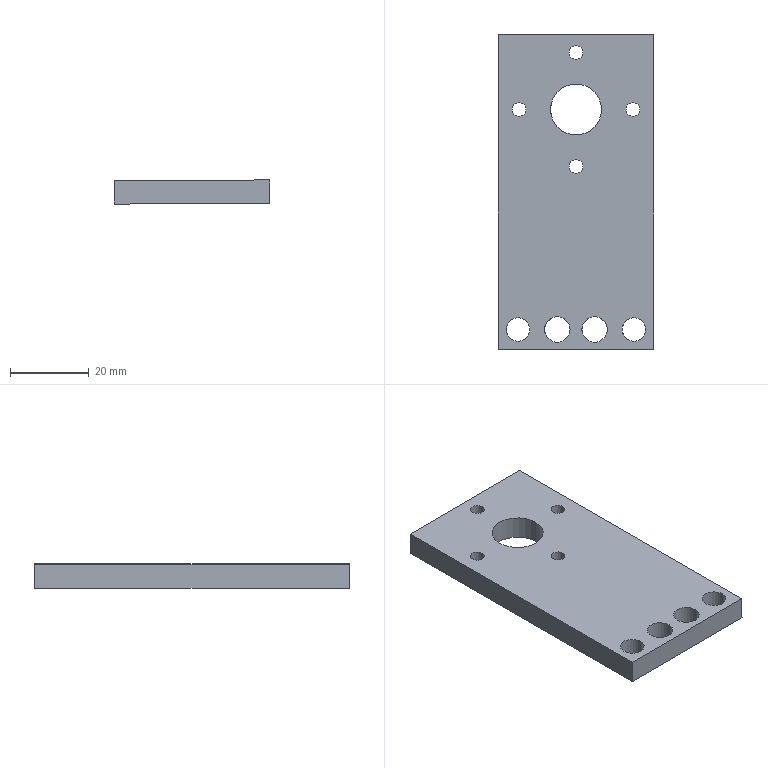Part | SolidWorks | features Cut 2, HoleWzd 2, Extrusion 1 | 1 solid | 24 faces | box 39.504 x 80 x 6.135 mm | volume 17187 mm3 | cylinder 18 | plane 6 | commonest cylinder face diameters 3.5 x8 6 x4 6.5 x4 13 x2
STEP:
#1=CARTESIAN_POINT('',(-183.995,65.629,-9.921));
#2=VERTEX_POINT('',#1);
#3=CARTESIAN_POINT('',(-187.495,65.629,-9.933));
#4=VERTEX_POINT('',#3);
#5=CARTESIAN_POINT('',(-185.745,65.629,-9.927));
#6=DIRECTION('',(0.003428,0.,-1.));
#7=DIRECTION('',(-1.,0.,-0.003428));
#8=AXIS2_PLACEMENT_3D('',#5,#6,#7);
#9=CIRCLE('',#8,1.75);
#10=EDGE_CURVE('',#2,#4,#9,.T.);
#11=ORIENTED_EDGE('',*,*,#10,.T.);
#12=CARTESIAN_POINT('',(-187.515,65.629,-3.933));
#13=VERTEX_POINT('',#12);
#14=CARTESIAN_POINT('',(-187.515,65.629,-3.933));
#15=DIRECTION('',(-0.003428,0.,1.));
#16=VECTOR('',#15,1000.);
#17=LINE('',#14,#16);
#18=EDGE_CURVE('',#4,#13,#17,.T.);
#19=ORIENTED_EDGE('',*,*,#18,.T.);
#20=CARTESIAN_POINT('',(-184.015,65.629,-3.921));
#21=VERTEX_POINT('',#20);
#22=CARTESIAN_POINT('',(-185.765,65.629,-3.927));
#23=DIRECTION('',(-0.003428,0.,1.));
#24=DIRECTION('',(1.,0.,0.003428));
#25=AXIS2_PLACEMENT_3D('',#22,#23,#24);
#26=CIRCLE('',#25,1.75);
#27=EDGE_CURVE('',#13,#21,#26,.T.);
#28=ORIENTED_EDGE('',*,*,#27,.T.);
#29=CARTESIAN_POINT('',(-184.015,65.629,-3.921));
#30=DIRECTION('',(-0.003428,0.,1.));
#31=VECTOR('',#30,1000.);
#32=LINE('',#29,#31);
#33=EDGE_CURVE('',#2,#21,#32,.T.);
#34=ORIENTED_EDGE('',*,*,#33,.F.);
#35=EDGE_LOOP('',(#11,#19,#28,#34));
#36=FACE_OUTER_BOUND('',#35,.T.);
#37=CARTESIAN_POINT('',(-185.765,65.629,-3.927));
#38=DIRECTION('',(-0.003428,0.,1.));
#39=DIRECTION('',(1.,0.,0.003428));
#40=AXIS2_PLACEMENT_3D('',#37,#38,#39);
#41=CYLINDRICAL_SURFACE('',#40,1.75);
#42=ADVANCED_FACE('',(#36),#41,.F.);
#43=CARTESIAN_POINT('',(-169.495,51.129,-9.871));
#44=VERTEX_POINT('',#43);
#45=CARTESIAN_POINT('',(-172.995,51.129,-9.883));
#46=VERTEX_POINT('',#45);
#47=CARTESIAN_POINT('',(-171.245,51.129,-9.877));
#48=DIRECTION('',(0.003428,0.,-1.));
#49=DIRECTION('',(-1.,0.,-0.003428));
#50=AXIS2_PLACEMENT_3D('',#47,#48,#49);
#51=CIRCLE('',#50,1.75);
#52=EDGE_CURVE('',#44,#46,#51,.T.);
#53=ORIENTED_EDGE('',*,*,#52,.T.);
#54=CARTESIAN_POINT('',(-173.015,51.129,-3.883));
#55=VERTEX_POINT('',#54);
#56=CARTESIAN_POINT('',(-173.015,51.129,-3.883));
#57=DIRECTION('',(-0.003428,0.,1.));
#58=VECTOR('',#57,1000.);
#59=LINE('',#56,#58);
#60=EDGE_CURVE('',#46,#55,#59,.T.);
#61=ORIENTED_EDGE('',*,*,#60,.T.);
#62=CARTESIAN_POINT('',(-169.515,51.129,-3.871));
#63=VERTEX_POINT('',#62);
#64=CARTESIAN_POINT('',(-171.265,51.129,-3.877));
#65=DIRECTION('',(-0.003428,0.,1.));
#66=DIRECTION('',(1.,0.,0.003428));
#67=AXIS2_PLACEMENT_3D('',#64,#65,#66);
#68=CIRCLE('',#67,1.75);
#69=EDGE_CURVE('',#55,#63,#68,.T.);
#70=ORIENTED_EDGE('',*,*,#69,.T.);
#71=CARTESIAN_POINT('',(-169.515,51.129,-3.871));
#72=DIRECTION('',(-0.003428,0.,1.));
#73=VECTOR('',#72,1000.);
#74=LINE('',#71,#73);
#75=EDGE_CURVE('',#44,#63,#74,.T.);
#76=ORIENTED_EDGE('',*,*,#75,.F.);
#77=EDGE_LOOP('',(#53,#61,#70,#76));
#78=FACE_OUTER_BOUND('',#77,.T.);
#79=CARTESIAN_POINT('',(-171.265,51.129,-3.877));
#80=DIRECTION('',(-0.003428,0.,1.));
#81=DIRECTION('',(1.,0.,0.003428));
#82=AXIS2_PLACEMENT_3D('',#79,#80,#81);
#83=CYLINDRICAL_SURFACE('',#82,1.75);
#84=ADVANCED_FACE('',(#78),#83,.F.);
#85=CARTESIAN_POINT('',(-183.995,36.629,-9.921));
#86=VERTEX_POINT('',#85);
#87=CARTESIAN_POINT('',(-187.495,36.629,-9.933));
#88=VERTEX_POINT('',#87);
#89=CARTESIAN_POINT('',(-185.745,36.629,-9.927));
#90=DIRECTION('',(0.003428,0.,-1.));
#91=DIRECTION('',(-1.,0.,-0.003428));
#92=AXIS2_PLACEMENT_3D('',#89,#90,#91);
#93=CIRCLE('',#92,1.75);
#94=EDGE_CURVE('',#86,#88,#93,.T.);
#95=ORIENTED_EDGE('',*,*,#94,.T.);
#96=CARTESIAN_POINT('',(-187.515,36.629,-3.933));
#97=VERTEX_POINT('',#96);
#98=CARTESIAN_POINT('',(-187.515,36.629,-3.933));
#99=DIRECTION('',(-0.003428,0.,1.));
#100=VECTOR('',#99,1000.);
#101=LINE('',#98,#100);
#102=EDGE_CURVE('',#88,#97,#101,.T.);
#103=ORIENTED_EDGE('',*,*,#102,.T.);
#104=CARTESIAN_POINT('',(-184.015,36.629,-3.921));
#105=VERTEX_POINT('',#104);
#106=CARTESIAN_POINT('',(-185.765,36.629,-3.927));
#107=DIRECTION('',(-0.003428,0.,1.));
#108=DIRECTION('',(1.,0.,0.003428));
#109=AXIS2_PLACEMENT_3D('',#106,#107,#108);
#110=CIRCLE('',#109,1.75);
#111=EDGE_CURVE('',#97,#105,#110,.T.);
#112=ORIENTED_EDGE('',*,*,#111,.T.);
#113=CARTESIAN_POINT('',(-184.015,36.629,-3.921));
#114=DIRECTION('',(-0.003428,0.,1.));
#115=VECTOR('',#114,1000.);
#116=LINE('',#113,#115);
#117=EDGE_CURVE('',#86,#105,#116,.T.);
#118=ORIENTED_EDGE('',*,*,#117,.F.);
#119=EDGE_LOOP('',(#95,#103,#112,#118));
#120=FACE_OUTER_BOUND('',#119,.T.);
#121=CARTESIAN_POINT('',(-185.765,36.629,-3.927));
#122=DIRECTION('',(-0.003428,0.,1.));
#123=DIRECTION('',(1.,0.,0.003428));
#124=AXIS2_PLACEMENT_3D('',#121,#122,#123);
#125=CYLINDRICAL_SURFACE('',#124,1.75);
#126=ADVANCED_FACE('',(#120),#125,.F.);
#127=CARTESIAN_POINT('',(-198.495,51.129,-9.97));
#128=VERTEX_POINT('',#127);
#129=CARTESIAN_POINT('',(-201.995,51.129,-9.982));
#130=VERTEX_POINT('',#129);
#131=CARTESIAN_POINT('',(-200.245,51.129,-9.976));
#132=DIRECTION('',(0.003428,0.,-1.));
#133=DIRECTION('',(-1.,0.,-0.003428));
#134=AXIS2_PLACEMENT_3D('',#131,#132,#133);
#135=CIRCLE('',#134,1.75);
#136=EDGE_CURVE('',#128,#130,#135,.T.);
#137=ORIENTED_EDGE('',*,*,#136,.T.);
#138=CARTESIAN_POINT('',(-202.015,51.129,-3.982));
#139=VERTEX_POINT('',#138);
#140=CARTESIAN_POINT('',(-202.015,51.129,-3.982));
#141=DIRECTION('',(-0.003428,0.,1.));
#142=VECTOR('',#141,1000.);
#143=LINE('',#140,#142);
#144=EDGE_CURVE('',#130,#139,#143,.T.);
#145=ORIENTED_EDGE('',*,*,#144,.T.);
#146=CARTESIAN_POINT('',(-198.515,51.129,-3.97));
#147=VERTEX_POINT('',#146);
#148=CARTESIAN_POINT('',(-200.265,51.129,-3.976));
#149=DIRECTION('',(-0.003428,0.,1.));
#150=DIRECTION('',(1.,0.,0.003428));
#151=AXIS2_PLACEMENT_3D('',#148,#149,#150);
#152=CIRCLE('',#151,1.75);
#153=EDGE_CURVE('',#139,#147,#152,.T.);
#154=ORIENTED_EDGE('',*,*,#153,.T.);
#155=CARTESIAN_POINT('',(-198.515,51.129,-3.97));
#156=DIRECTION('',(-0.003428,0.,1.));
#157=VECTOR('',#156,1000.);
#158=LINE('',#155,#157);
#159=EDGE_CURVE('',#128,#147,#158,.T.);
#160=ORIENTED_EDGE('',*,*,#159,.F.);
#161=EDGE_LOOP('',(#137,#145,#154,#160));
#162=FACE_OUTER_BOUND('',#161,.T.);
#163=CARTESIAN_POINT('',(-200.265,51.129,-3.976));
#164=DIRECTION('',(-0.003428,0.,1.));
#165=DIRECTION('',(1.,0.,0.003428));
#166=AXIS2_PLACEMENT_3D('',#163,#164,#165);
#167=CYLINDRICAL_SURFACE('',#166,1.75);
#168=ADVANCED_FACE('',(#162),#167,.F.);
#169=CARTESIAN_POINT('',(-179.265,51.129,-3.904));
#170=VERTEX_POINT('',#169);
#171=CARTESIAN_POINT('',(-192.265,51.129,-3.949));
#172=VERTEX_POINT('',#171);
#173=CARTESIAN_POINT('',(-185.765,51.129,-3.927));
#174=DIRECTION('',(0.003428,0.,-1.));
#175=DIRECTION('',(-1.,0.,-0.003428));
#176=AXIS2_PLACEMENT_3D('',#173,#174,#175);
#177=CIRCLE('',#176,6.5);
#178=EDGE_CURVE('',#170,#172,#177,.T.);
#179=ORIENTED_EDGE('',*,*,#178,.F.);
#180=CARTESIAN_POINT('',(-179.245,51.129,-9.904));
#181=VERTEX_POINT('',#180);
#182=CARTESIAN_POINT('',(-179.266,51.129,-3.769));
#183=DIRECTION('',(0.003428,0.,-1.));
#184=VECTOR('',#183,1000.);
#185=LINE('',#182,#184);
#186=EDGE_CURVE('',#170,#181,#185,.T.);
#187=ORIENTED_EDGE('',*,*,#186,.T.);
#188=CARTESIAN_POINT('',(-192.245,51.129,-9.949));
#189=VERTEX_POINT('',#188);
#190=CARTESIAN_POINT('',(-185.745,51.129,-9.927));
#191=DIRECTION('',(0.003428,0.,-1.));
#192=DIRECTION('',(-1.,0.,-0.003428));
#193=AXIS2_PLACEMENT_3D('',#190,#191,#192);
#194=CIRCLE('',#193,6.5);
#195=EDGE_CURVE('',#181,#189,#194,.T.);
#196=ORIENTED_EDGE('',*,*,#195,.T.);
#197=CARTESIAN_POINT('',(-192.266,51.129,-3.814));
#198=DIRECTION('',(0.003428,0.,-1.));
#199=VECTOR('',#198,1000.);
#200=LINE('',#197,#199);
#201=EDGE_CURVE('',#172,#189,#200,.T.);
#202=ORIENTED_EDGE('',*,*,#201,.F.);
#203=EDGE_LOOP('',(#179,#187,#196,#202));
#204=FACE_OUTER_BOUND('',#203,.T.);
#205=CARTESIAN_POINT('',(-185.766,51.129,-3.791));
#206=DIRECTION('',(0.003428,0.,-1.));
#207=DIRECTION('',(-1.,0.,-0.003428));
#208=AXIS2_PLACEMENT_3D('',#205,#206,#207);
#209=CYLINDRICAL_SURFACE('',#208,6.5);
#210=ADVANCED_FACE('',(#204),#209,.F.);
#211=CARTESIAN_POINT('',(-187.238,-4.871,-9.932));
#212=VERTEX_POINT('',#211);
#213=CARTESIAN_POINT('',(-193.738,-4.871,-9.954));
#214=VERTEX_POINT('',#213);
#215=CARTESIAN_POINT('',(-190.488,-4.871,-9.943));
#216=DIRECTION('',(0.003428,0.,-1.));
#217=DIRECTION('',(-1.,0.,-0.003428));
#218=AXIS2_PLACEMENT_3D('',#215,#216,#217);
#219=CIRCLE('',#218,3.25);
#220=EDGE_CURVE('',#212,#214,#219,.T.);
#221=ORIENTED_EDGE('',*,*,#220,.T.);
#222=CARTESIAN_POINT('',(-193.758,-4.871,-3.954));
#223=VERTEX_POINT('',#222);
#224=CARTESIAN_POINT('',(-193.758,-4.871,-3.954));
#225=DIRECTION('',(-0.003428,0.,1.));
#226=VECTOR('',#225,1000.);
#227=LINE('',#224,#226);
#228=EDGE_CURVE('',#214,#223,#227,.T.);
#229=ORIENTED_EDGE('',*,*,#228,.T.);
#230=CARTESIAN_POINT('',(-187.258,-4.871,-3.932));
#231=VERTEX_POINT('',#230);
#232=CARTESIAN_POINT('',(-190.508,-4.871,-3.943));
#233=DIRECTION('',(-0.003428,0.,1.));
#234=DIRECTION('',(1.,0.,0.003428));
#235=AXIS2_PLACEMENT_3D('',#232,#233,#234);
#236=CIRCLE('',#235,3.25);
#237=EDGE_CURVE('',#223,#231,#236,.T.);
#238=ORIENTED_EDGE('',*,*,#237,.T.);
#239=CARTESIAN_POINT('',(-187.258,-4.871,-3.932));
#240=DIRECTION('',(-0.003428,0.,1.));
#241=VECTOR('',#240,1000.);
#242=LINE('',#239,#241);
#243=EDGE_CURVE('',#212,#231,#242,.T.);
#244=ORIENTED_EDGE('',*,*,#243,.F.);
#245=EDGE_LOOP('',(#221,#229,#238,#244));
#246=FACE_OUTER_BOUND('',#245,.T.);
#247=CARTESIAN_POINT('',(-190.508,-4.871,-3.943));
#248=DIRECTION('',(-0.003428,0.,1.));
#249=DIRECTION('',(1.,0.,0.003428));
#250=AXIS2_PLACEMENT_3D('',#247,#248,#249);
#251=CYLINDRICAL_SURFACE('',#250,3.25);
#252=ADVANCED_FACE('',(#246),#251,.F.);
#253=CARTESIAN_POINT('',(-177.754,-4.871,-9.899));
#254=VERTEX_POINT('',#253);
#255=CARTESIAN_POINT('',(-184.254,-4.871,-9.922));
#256=VERTEX_POINT('',#255);
#257=CARTESIAN_POINT('',(-181.004,-4.871,-9.91));
#258=DIRECTION('',(0.003428,0.,-1.));
#259=DIRECTION('',(-1.,0.,-0.003428));
#260=AXIS2_PLACEMENT_3D('',#257,#258,#259);
#261=CIRCLE('',#260,3.25);
#262=EDGE_CURVE('',#254,#256,#261,.T.);
#263=ORIENTED_EDGE('',*,*,#262,.T.);
#264=CARTESIAN_POINT('',(-184.275,-4.871,-3.922));
#265=VERTEX_POINT('',#264);
#266=CARTESIAN_POINT('',(-184.275,-4.871,-3.922));
#267=DIRECTION('',(-0.003428,0.,1.));
#268=VECTOR('',#267,1000.);
#269=LINE('',#266,#268);
#270=EDGE_CURVE('',#256,#265,#269,.T.);
#271=ORIENTED_EDGE('',*,*,#270,.T.);
#272=CARTESIAN_POINT('',(-177.775,-4.871,-3.899));
#273=VERTEX_POINT('',#272);
#274=CARTESIAN_POINT('',(-181.025,-4.871,-3.91));
#275=DIRECTION('',(-0.003428,0.,1.));
#276=DIRECTION('',(1.,0.,0.003428));
#277=AXIS2_PLACEMENT_3D('',#274,#275,#276);
#278=CIRCLE('',#277,3.25);
#279=EDGE_CURVE('',#265,#273,#278,.T.);
#280=ORIENTED_EDGE('',*,*,#279,.T.);
#281=CARTESIAN_POINT('',(-177.775,-4.871,-3.899));
#282=DIRECTION('',(-0.003428,0.,1.));
#283=VECTOR('',#282,1000.);
#284=LINE('',#281,#283);
#285=EDGE_CURVE('',#254,#273,#284,.T.);
#286=ORIENTED_EDGE('',*,*,#285,.F.);
#287=EDGE_LOOP('',(#263,#271,#280,#286));
#288=FACE_OUTER_BOUND('',#287,.T.);
#289=CARTESIAN_POINT('',(-181.025,-4.871,-3.91));
#290=DIRECTION('',(-0.003428,0.,1.));
#291=DIRECTION('',(1.,0.,0.003428));
#292=AXIS2_PLACEMENT_3D('',#289,#290,#291);
#293=CYLINDRICAL_SURFACE('',#292,3.25);
#294=ADVANCED_FACE('',(#288),#293,.F.);
#295=CARTESIAN_POINT('',(-168.004,-4.871,-9.866));
#296=VERTEX_POINT('',#295);
#297=CARTESIAN_POINT('',(-174.004,-4.871,-9.886));
#298=VERTEX_POINT('',#297);
#299=CARTESIAN_POINT('',(-171.004,-4.871,-9.876));
#300=DIRECTION('',(0.003428,0.,-1.));
#301=DIRECTION('',(-1.,0.,-0.003428));
#302=AXIS2_PLACEMENT_3D('',#299,#300,#301);
#303=CIRCLE('',#302,3.);
#304=EDGE_CURVE('',#296,#298,#303,.T.);
#305=ORIENTED_EDGE('',*,*,#304,.T.);
#306=CARTESIAN_POINT('',(-174.025,-4.871,-3.886));
#307=VERTEX_POINT('',#306);
#308=CARTESIAN_POINT('',(-173.991,-4.871,-13.886));
#309=DIRECTION('',(-0.003428,0.,1.));
#310=VECTOR('',#309,1000.);
#311=LINE('',#308,#310);
#312=EDGE_CURVE('',#298,#307,#311,.T.);
#313=ORIENTED_EDGE('',*,*,#312,.T.);
#314=CARTESIAN_POINT('',(-168.025,-4.871,-3.866));
#315=VERTEX_POINT('',#314);
#316=CARTESIAN_POINT('',(-171.025,-4.871,-3.876));
#317=DIRECTION('',(-0.003428,0.,1.));
#318=DIRECTION('',(1.,0.,0.003428));
#319=AXIS2_PLACEMENT_3D('',#316,#317,#318);
#320=CIRCLE('',#319,3.);
#321=EDGE_CURVE('',#307,#315,#320,.T.);
#322=ORIENTED_EDGE('',*,*,#321,.T.);
#323=CARTESIAN_POINT('',(-167.991,-4.871,-13.866));
#324=DIRECTION('',(-0.003428,0.,1.));
#325=VECTOR('',#324,1000.);
#326=LINE('',#323,#325);
#327=EDGE_CURVE('',#296,#315,#326,.T.);
#328=ORIENTED_EDGE('',*,*,#327,.F.);
#329=EDGE_LOOP('',(#305,#313,#322,#328));
#330=FACE_OUTER_BOUND('',#329,.T.);
#331=CARTESIAN_POINT('',(-170.991,-4.871,-13.876));
#332=DIRECTION('',(-0.003428,0.,1.));
#333=DIRECTION('',(1.,0.,0.003428));
#334=AXIS2_PLACEMENT_3D('',#331,#332,#333);
#335=CYLINDRICAL_SURFACE('',#334,3.);
#336=ADVANCED_FACE('',(#330),#335,.F.);
#337=CARTESIAN_POINT('',(-197.487,-4.871,-9.967));
#338=VERTEX_POINT('',#337);
#339=CARTESIAN_POINT('',(-203.487,-4.871,-9.988));
#340=VERTEX_POINT('',#339);
#341=CARTESIAN_POINT('',(-200.487,-4.871,-9.977));
#342=DIRECTION('',(0.003428,0.,-1.));
#343=DIRECTION('',(-1.,0.,-0.003428));
#344=AXIS2_PLACEMENT_3D('',#341,#342,#343);
#345=CIRCLE('',#344,3.);
#346=EDGE_CURVE('',#338,#340,#345,.T.);
#347=ORIENTED_EDGE('',*,*,#346,.T.);
#348=CARTESIAN_POINT('',(-203.508,-4.871,-3.988));
#349=VERTEX_POINT('',#348);
#350=CARTESIAN_POINT('',(-203.474,-4.871,-13.987));
#351=DIRECTION('',(-0.003428,0.,1.));
#352=VECTOR('',#351,1000.);
#353=LINE('',#350,#352);
#354=EDGE_CURVE('',#340,#349,#353,.T.);
#355=ORIENTED_EDGE('',*,*,#354,.T.);
#356=CARTESIAN_POINT('',(-197.508,-4.871,-3.967));
#357=VERTEX_POINT('',#356);
#358=CARTESIAN_POINT('',(-200.508,-4.871,-3.977));
#359=DIRECTION('',(-0.003428,0.,1.));
#360=DIRECTION('',(1.,0.,0.003428));
#361=AXIS2_PLACEMENT_3D('',#358,#359,#360);
#362=CIRCLE('',#361,3.);
#363=EDGE_CURVE('',#349,#357,#362,.T.);
#364=ORIENTED_EDGE('',*,*,#363,.T.);
#365=CARTESIAN_POINT('',(-197.474,-4.871,-13.967));
#366=DIRECTION('',(-0.003428,0.,1.));
#367=VECTOR('',#366,1000.);
#368=LINE('',#365,#367);
#369=EDGE_CURVE('',#338,#357,#368,.T.);
#370=ORIENTED_EDGE('',*,*,#369,.F.);
#371=EDGE_LOOP('',(#347,#355,#364,#370));
#372=FACE_OUTER_BOUND('',#371,.T.);
#373=CARTESIAN_POINT('',(-200.474,-4.871,-13.977));
#374=DIRECTION('',(-0.003428,0.,1.));
#375=DIRECTION('',(1.,0.,0.003428));
#376=AXIS2_PLACEMENT_3D('',#373,#374,#375);
#377=CYLINDRICAL_SURFACE('',#376,3.);
#378=ADVANCED_FACE('',(#372),#377,.F.);
#379=CARTESIAN_POINT('',(-166.004,-9.871,-9.859));
#380=VERTEX_POINT('',#379);
#381=CARTESIAN_POINT('',(-166.004,70.129,-9.859));
#382=VERTEX_POINT('',#381);
#383=CARTESIAN_POINT('',(-166.004,-9.871,-9.859));
#384=DIRECTION('',(0.,1.,0.));
#385=VECTOR('',#384,1000.);
#386=LINE('',#383,#385);
#387=EDGE_CURVE('',#380,#382,#386,.T.);
#388=ORIENTED_EDGE('',*,*,#387,.T.);
#389=CARTESIAN_POINT('',(-166.025,70.129,-3.859));
#390=VERTEX_POINT('',#389);
#391=CARTESIAN_POINT('',(-166.025,70.129,-3.859));
#392=DIRECTION('',(0.003428,0.,-1.));
#393=VECTOR('',#392,1000.);
#394=LINE('',#391,#393);
#395=EDGE_CURVE('',#390,#382,#394,.T.);
#396=ORIENTED_EDGE('',*,*,#395,.F.);
#397=CARTESIAN_POINT('',(-166.025,-9.871,-3.859));
#398=VERTEX_POINT('',#397);
#399=CARTESIAN_POINT('',(-166.025,-9.871,-3.859));
#400=DIRECTION('',(0.,1.,0.));
#401=VECTOR('',#400,1000.);
#402=LINE('',#399,#401);
#403=EDGE_CURVE('',#398,#390,#402,.T.);
#404=ORIENTED_EDGE('',*,*,#403,.F.);
#405=CARTESIAN_POINT('',(-166.025,-9.871,-3.859));
#406=DIRECTION('',(0.003428,0.,-1.));
#407=VECTOR('',#406,1000.);
#408=LINE('',#405,#407);
#409=EDGE_CURVE('',#398,#380,#408,.T.);
#410=ORIENTED_EDGE('',*,*,#409,.T.);
#411=EDGE_LOOP('',(#388,#396,#404,#410));
#412=FACE_OUTER_BOUND('',#411,.T.);
#413=CARTESIAN_POINT('',(-166.025,-9.871,-3.859));
#414=DIRECTION('',(-1.,0.,-0.003428));
#415=DIRECTION('',(-0.003428,0.,1.));
#416=AXIS2_PLACEMENT_3D('',#413,#414,#415);
#417=PLANE('',#416);
#418=ADVANCED_FACE('',(#412),#417,.F.);
#419=CARTESIAN_POINT('',(-205.487,70.129,-9.994));
#420=VERTEX_POINT('',#419);
#421=CARTESIAN_POINT('',(-205.487,70.129,-9.994));
#422=DIRECTION('',(-1.,0.,-0.003428));
#423=VECTOR('',#422,1000.);
#424=LINE('',#421,#423);
#425=EDGE_CURVE('',#382,#420,#424,.T.);
#426=ORIENTED_EDGE('',*,*,#425,.T.);
#427=CARTESIAN_POINT('',(-205.508,70.129,-3.994));
#428=VERTEX_POINT('',#427);
#429=CARTESIAN_POINT('',(-205.508,70.129,-3.994));
#430=DIRECTION('',(0.003428,0.,-1.));
#431=VECTOR('',#430,1000.);
#432=LINE('',#429,#431);
#433=EDGE_CURVE('',#428,#420,#432,.T.);
#434=ORIENTED_EDGE('',*,*,#433,.F.);
#435=CARTESIAN_POINT('',(-205.508,70.129,-3.994));
#436=DIRECTION('',(-1.,0.,-0.003428));
#437=VECTOR('',#436,1000.);
#438=LINE('',#435,#437);
#439=EDGE_CURVE('',#390,#428,#438,.T.);
#440=ORIENTED_EDGE('',*,*,#439,.F.);
#441=ORIENTED_EDGE('',*,*,#395,.T.);
#442=EDGE_LOOP('',(#426,#434,#440,#441));
#443=FACE_OUTER_BOUND('',#442,.T.);
#444=CARTESIAN_POINT('',(-205.508,70.129,-3.994));
#445=DIRECTION('',(0.,-1.,0.));
#446=DIRECTION('',(0.,0.,-1.));
#447=AXIS2_PLACEMENT_3D('',#444,#445,#446);
#448=PLANE('',#447);
#449=ADVANCED_FACE('',(#443),#448,.F.);
#450=CARTESIAN_POINT('',(-205.487,-9.871,-9.994));
#451=VERTEX_POINT('',#450);
#452=CARTESIAN_POINT('',(-205.487,-9.871,-9.994));
#453=DIRECTION('',(0.,-1.,0.));
#454=VECTOR('',#453,1000.);
#455=LINE('',#452,#454);
#456=EDGE_CURVE('',#420,#451,#455,.T.);
#457=ORIENTED_EDGE('',*,*,#456,.T.);
#458=CARTESIAN_POINT('',(-205.508,-9.871,-3.994));
#459=VERTEX_POINT('',#458);
#460=CARTESIAN_POINT('',(-205.508,-9.871,-3.994));
#461=DIRECTION('',(0.003428,0.,-1.));
#462=VECTOR('',#461,1000.);
#463=LINE('',#460,#462);
#464=EDGE_CURVE('',#459,#451,#463,.T.);
#465=ORIENTED_EDGE('',*,*,#464,.F.);
#466=CARTESIAN_POINT('',(-205.508,-9.871,-3.994));
#467=DIRECTION('',(0.,-1.,0.));
#468=VECTOR('',#467,1000.);
#469=LINE('',#466,#468);
#470=EDGE_CURVE('',#428,#459,#469,.T.);
#471=ORIENTED_EDGE('',*,*,#470,.F.);
#472=ORIENTED_EDGE('',*,*,#433,.T.);
#473=EDGE_LOOP('',(#457,#465,#471,#472));
#474=FACE_OUTER_BOUND('',#473,.T.);
#475=CARTESIAN_POINT('',(-205.508,-9.871,-3.994));
#476=DIRECTION('',(1.,0.,0.003428));
#477=DIRECTION('',(0.003428,0.,-1.));
#478=AXIS2_PLACEMENT_3D('',#475,#476,#477);
#479=PLANE('',#478);
#480=ADVANCED_FACE('',(#474),#479,.F.);
#481=CARTESIAN_POINT('',(-205.487,-9.871,-9.994));
#482=DIRECTION('',(1.,0.,0.003428));
#483=VECTOR('',#482,1000.);
#484=LINE('',#481,#483);
#485=EDGE_CURVE('',#451,#380,#484,.T.);
#486=ORIENTED_EDGE('',*,*,#485,.T.);
#487=ORIENTED_EDGE('',*,*,#409,.F.);
#488=CARTESIAN_POINT('',(-205.508,-9.871,-3.994));
#489=DIRECTION('',(1.,0.,0.003428));
#490=VECTOR('',#489,1000.);
#491=LINE('',#488,#490);
#492=EDGE_CURVE('',#459,#398,#491,.T.);
#493=ORIENTED_EDGE('',*,*,#492,.F.);
#494=ORIENTED_EDGE('',*,*,#464,.T.);
#495=EDGE_LOOP('',(#486,#487,#493,#494));
#496=FACE_OUTER_BOUND('',#495,.T.);
#497=CARTESIAN_POINT('',(-205.508,-9.871,-3.994));
#498=DIRECTION('',(0.,1.,0.));
#499=DIRECTION('',(0.,0.,1.));
#500=AXIS2_PLACEMENT_3D('',#497,#498,#499);
#501=PLANE('',#500);
#502=ADVANCED_FACE('',(#496),#501,.F.);
#503=CARTESIAN_POINT('',(-185.765,65.629,-3.927));
#504=DIRECTION('',(-0.003428,0.,1.));
#505=DIRECTION('',(1.,0.,0.003428));
#506=AXIS2_PLACEMENT_3D('',#503,#504,#505);
#507=CIRCLE('',#506,1.75);
#508=EDGE_CURVE('',#21,#13,#507,.T.);
#509=ORIENTED_EDGE('',*,*,#508,.F.);
#510=ORIENTED_EDGE('',*,*,#27,.F.);
#511=EDGE_LOOP('',(#509,#510));
#512=FACE_BOUND('',#511,.T.);
#513=CARTESIAN_POINT('',(-171.265,51.129,-3.877));
#514=DIRECTION('',(-0.003428,0.,1.));
#515=DIRECTION('',(1.,0.,0.003428));
#516=AXIS2_PLACEMENT_3D('',#513,#514,#515);
#517=CIRCLE('',#516,1.75);
#518=EDGE_CURVE('',#63,#55,#517,.T.);
#519=ORIENTED_EDGE('',*,*,#518,.F.);
#520=ORIENTED_EDGE('',*,*,#69,.F.);
#521=EDGE_LOOP('',(#519,#520));
#522=FACE_BOUND('',#521,.T.);
#523=CARTESIAN_POINT('',(-185.765,36.629,-3.927));
#524=DIRECTION('',(-0.003428,0.,1.));
#525=DIRECTION('',(1.,0.,0.003428));
#526=AXIS2_PLACEMENT_3D('',#523,#524,#525);
#527=CIRCLE('',#526,1.75);
#528=EDGE_CURVE('',#105,#97,#527,.T.);
#529=ORIENTED_EDGE('',*,*,#528,.F.);
#530=ORIENTED_EDGE('',*,*,#111,.F.);
#531=EDGE_LOOP('',(#529,#530));
#532=FACE_BOUND('',#531,.T.);
#533=CARTESIAN_POINT('',(-200.265,51.129,-3.976));
#534=DIRECTION('',(-0.003428,0.,1.));
#535=DIRECTION('',(1.,0.,0.003428));
#536=AXIS2_PLACEMENT_3D('',#533,#534,#535);
#537=CIRCLE('',#536,1.75);
#538=EDGE_CURVE('',#147,#139,#537,.T.);
#539=ORIENTED_EDGE('',*,*,#538,.F.);
#540=ORIENTED_EDGE('',*,*,#153,.F.);
#541=EDGE_LOOP('',(#539,#540));
#542=FACE_BOUND('',#541,.T.);
#543=CARTESIAN_POINT('',(-185.765,51.129,-3.927));
#544=DIRECTION('',(0.003428,0.,-1.));
#545=DIRECTION('',(-1.,0.,-0.003428));
#546=AXIS2_PLACEMENT_3D('',#543,#544,#545);
#547=CIRCLE('',#546,6.5);
#548=EDGE_CURVE('',#172,#170,#547,.T.);
#549=ORIENTED_EDGE('',*,*,#548,.T.);
#550=ORIENTED_EDGE('',*,*,#178,.T.);
#551=EDGE_LOOP('',(#549,#550));
#552=FACE_BOUND('',#551,.T.);
#553=CARTESIAN_POINT('',(-190.508,-4.871,-3.943));
#554=DIRECTION('',(-0.003428,0.,1.));
#555=DIRECTION('',(1.,0.,0.003428));
#556=AXIS2_PLACEMENT_3D('',#553,#554,#555);
#557=CIRCLE('',#556,3.25);
#558=EDGE_CURVE('',#231,#223,#557,.T.);
#559=ORIENTED_EDGE('',*,*,#558,.F.);
#560=ORIENTED_EDGE('',*,*,#237,.F.);
#561=EDGE_LOOP('',(#559,#560));
#562=FACE_BOUND('',#561,.T.);
#563=CARTESIAN_POINT('',(-181.025,-4.871,-3.91));
#564=DIRECTION('',(-0.003428,0.,1.));
#565=DIRECTION('',(1.,0.,0.003428));
#566=AXIS2_PLACEMENT_3D('',#563,#564,#565);
#567=CIRCLE('',#566,3.25);
#568=EDGE_CURVE('',#273,#265,#567,.T.);
#569=ORIENTED_EDGE('',*,*,#568,.F.);
#570=ORIENTED_EDGE('',*,*,#279,.F.);
#571=EDGE_LOOP('',(#569,#570));
#572=FACE_BOUND('',#571,.T.);
#573=CARTESIAN_POINT('',(-171.025,-4.871,-3.876));
#574=DIRECTION('',(-0.003428,0.,1.));
#575=DIRECTION('',(1.,0.,0.003428));
#576=AXIS2_PLACEMENT_3D('',#573,#574,#575);
#577=CIRCLE('',#576,3.);
#578=EDGE_CURVE('',#315,#307,#577,.T.);
#579=ORIENTED_EDGE('',*,*,#578,.F.);
#580=ORIENTED_EDGE('',*,*,#321,.F.);
#581=EDGE_LOOP('',(#579,#580));
#582=FACE_BOUND('',#581,.T.);
#583=CARTESIAN_POINT('',(-200.508,-4.871,-3.977));
#584=DIRECTION('',(-0.003428,0.,1.));
#585=DIRECTION('',(1.,0.,0.003428));
#586=AXIS2_PLACEMENT_3D('',#583,#584,#585);
#587=CIRCLE('',#586,3.);
#588=EDGE_CURVE('',#357,#349,#587,.T.);
#589=ORIENTED_EDGE('',*,*,#588,.F.);
#590=ORIENTED_EDGE('',*,*,#363,.F.);
#591=EDGE_LOOP('',(#589,#590));
#592=FACE_BOUND('',#591,.T.);
#593=ORIENTED_EDGE('',*,*,#403,.T.);
#594=ORIENTED_EDGE('',*,*,#439,.T.);
#595=ORIENTED_EDGE('',*,*,#470,.T.);
#596=ORIENTED_EDGE('',*,*,#492,.T.);
#597=EDGE_LOOP('',(#593,#594,#595,#596));
#598=FACE_OUTER_BOUND('',#597,.T.);
#599=CARTESIAN_POINT('',(0.01128,0.,-3.29));
#600=DIRECTION('',(0.003428,0.,-1.));
#601=DIRECTION('',(-1.,0.,-0.003428));
#602=AXIS2_PLACEMENT_3D('',#599,#600,#601);
#603=PLANE('',#602);
#604=ADVANCED_FACE('',(#512,#522,#532,#542,#552,#562,#572,#582,#592,#598),#603,.F.);
#605=ORIENTED_EDGE('',*,*,#10,.F.);
#606=CARTESIAN_POINT('',(-185.745,65.629,-9.927));
#607=DIRECTION('',(0.003428,0.,-1.));
#608=DIRECTION('',(-1.,0.,-0.003428));
#609=AXIS2_PLACEMENT_3D('',#606,#607,#608);
#610=CIRCLE('',#609,1.75);
#611=EDGE_CURVE('',#4,#2,#610,.T.);
#612=ORIENTED_EDGE('',*,*,#611,.F.);
#613=EDGE_LOOP('',(#605,#612));
#614=FACE_BOUND('',#613,.T.);
#615=ORIENTED_EDGE('',*,*,#52,.F.);
#616=CARTESIAN_POINT('',(-171.245,51.129,-9.877));
#617=DIRECTION('',(0.003428,0.,-1.));
#618=DIRECTION('',(-1.,0.,-0.003428));
#619=AXIS2_PLACEMENT_3D('',#616,#617,#618);
#620=CIRCLE('',#619,1.75);
#621=EDGE_CURVE('',#46,#44,#620,.T.);
#622=ORIENTED_EDGE('',*,*,#621,.F.);
#623=EDGE_LOOP('',(#615,#622));
#624=FACE_BOUND('',#623,.T.);
#625=ORIENTED_EDGE('',*,*,#94,.F.);
#626=CARTESIAN_POINT('',(-185.745,36.629,-9.927));
#627=DIRECTION('',(0.003428,0.,-1.));
#628=DIRECTION('',(-1.,0.,-0.003428));
#629=AXIS2_PLACEMENT_3D('',#626,#627,#628);
#630=CIRCLE('',#629,1.75);
#631=EDGE_CURVE('',#88,#86,#630,.T.);
#632=ORIENTED_EDGE('',*,*,#631,.F.);
#633=EDGE_LOOP('',(#625,#632));
#634=FACE_BOUND('',#633,.T.);
#635=ORIENTED_EDGE('',*,*,#136,.F.);
#636=CARTESIAN_POINT('',(-200.245,51.129,-9.976));
#637=DIRECTION('',(0.003428,0.,-1.));
#638=DIRECTION('',(-1.,0.,-0.003428));
#639=AXIS2_PLACEMENT_3D('',#636,#637,#638);
#640=CIRCLE('',#639,1.75);
#641=EDGE_CURVE('',#130,#128,#640,.T.);
#642=ORIENTED_EDGE('',*,*,#641,.F.);
#643=EDGE_LOOP('',(#635,#642));
#644=FACE_BOUND('',#643,.T.);
#645=CARTESIAN_POINT('',(-185.745,51.129,-9.927));
#646=DIRECTION('',(0.003428,0.,-1.));
#647=DIRECTION('',(-1.,0.,-0.003428));
#648=AXIS2_PLACEMENT_3D('',#645,#646,#647);
#649=CIRCLE('',#648,6.5);
#650=EDGE_CURVE('',#189,#181,#649,.T.);
#651=ORIENTED_EDGE('',*,*,#650,.F.);
#652=ORIENTED_EDGE('',*,*,#195,.F.);
#653=EDGE_LOOP('',(#651,#652));
#654=FACE_BOUND('',#653,.T.);
#655=ORIENTED_EDGE('',*,*,#220,.F.);
#656=CARTESIAN_POINT('',(-190.488,-4.871,-9.943));
#657=DIRECTION('',(0.003428,0.,-1.));
#658=DIRECTION('',(-1.,0.,-0.003428));
#659=AXIS2_PLACEMENT_3D('',#656,#657,#658);
#660=CIRCLE('',#659,3.25);
#661=EDGE_CURVE('',#214,#212,#660,.T.);
#662=ORIENTED_EDGE('',*,*,#661,.F.);
#663=EDGE_LOOP('',(#655,#662));
#664=FACE_BOUND('',#663,.T.);
#665=ORIENTED_EDGE('',*,*,#262,.F.);
#666=CARTESIAN_POINT('',(-181.004,-4.871,-9.91));
#667=DIRECTION('',(0.003428,0.,-1.));
#668=DIRECTION('',(-1.,0.,-0.003428));
#669=AXIS2_PLACEMENT_3D('',#666,#667,#668);
#670=CIRCLE('',#669,3.25);
#671=EDGE_CURVE('',#256,#254,#670,.T.);
#672=ORIENTED_EDGE('',*,*,#671,.F.);
#673=EDGE_LOOP('',(#665,#672));
#674=FACE_BOUND('',#673,.T.);
#675=ORIENTED_EDGE('',*,*,#304,.F.);
#676=CARTESIAN_POINT('',(-171.004,-4.871,-9.876));
#677=DIRECTION('',(0.003428,0.,-1.));
#678=DIRECTION('',(-1.,0.,-0.003428));
#679=AXIS2_PLACEMENT_3D('',#676,#677,#678);
#680=CIRCLE('',#679,3.);
#681=EDGE_CURVE('',#298,#296,#680,.T.);
#682=ORIENTED_EDGE('',*,*,#681,.F.);
#683=EDGE_LOOP('',(#675,#682));
#684=FACE_BOUND('',#683,.T.);
#685=ORIENTED_EDGE('',*,*,#346,.F.);
#686=CARTESIAN_POINT('',(-200.487,-4.871,-9.977));
#687=DIRECTION('',(0.003428,0.,-1.));
#688=DIRECTION('',(-1.,0.,-0.003428));
#689=AXIS2_PLACEMENT_3D('',#686,#687,#688);
#690=CIRCLE('',#689,3.);
#691=EDGE_CURVE('',#340,#338,#690,.T.);
#692=ORIENTED_EDGE('',*,*,#691,.F.);
#693=EDGE_LOOP('',(#685,#692));
#694=FACE_BOUND('',#693,.T.);
#695=ORIENTED_EDGE('',*,*,#387,.F.);
#696=ORIENTED_EDGE('',*,*,#485,.F.);
#697=ORIENTED_EDGE('',*,*,#456,.F.);
#698=ORIENTED_EDGE('',*,*,#425,.F.);
#699=EDGE_LOOP('',(#695,#696,#697,#698));
#700=FACE_OUTER_BOUND('',#699,.T.);
#701=CARTESIAN_POINT('',(0.03185,0.,-9.29));
#702=DIRECTION('',(0.003428,0.,-1.));
#703=DIRECTION('',(-1.,0.,-0.003428));
#704=AXIS2_PLACEMENT_3D('',#701,#702,#703);
#705=PLANE('',#704);
#706=ADVANCED_FACE('',(#614,#624,#634,#644,#654,#664,#674,#684,#694,#700),#705,.T.);
#707=ORIENTED_EDGE('',*,*,#354,.F.);
#708=ORIENTED_EDGE('',*,*,#691,.T.);
#709=ORIENTED_EDGE('',*,*,#369,.T.);
#710=ORIENTED_EDGE('',*,*,#588,.T.);
#711=EDGE_LOOP('',(#707,#708,#709,#710));
#712=FACE_OUTER_BOUND('',#711,.T.);
#713=CARTESIAN_POINT('',(-200.474,-4.871,-13.977));
#714=DIRECTION('',(-0.003428,0.,1.));
#715=DIRECTION('',(1.,0.,0.003428));
#716=AXIS2_PLACEMENT_3D('',#713,#714,#715);
#717=CYLINDRICAL_SURFACE('',#716,3.);
#718=ADVANCED_FACE('',(#712),#717,.F.);
#719=ORIENTED_EDGE('',*,*,#312,.F.);
#720=ORIENTED_EDGE('',*,*,#681,.T.);
#721=ORIENTED_EDGE('',*,*,#327,.T.);
#722=ORIENTED_EDGE('',*,*,#578,.T.);
#723=EDGE_LOOP('',(#719,#720,#721,#722));
#724=FACE_OUTER_BOUND('',#723,.T.);
#725=CARTESIAN_POINT('',(-170.991,-4.871,-13.876));
#726=DIRECTION('',(-0.003428,0.,1.));
#727=DIRECTION('',(1.,0.,0.003428));
#728=AXIS2_PLACEMENT_3D('',#725,#726,#727);
#729=CYLINDRICAL_SURFACE('',#728,3.);
#730=ADVANCED_FACE('',(#724),#729,.F.);
#731=ORIENTED_EDGE('',*,*,#270,.F.);
#732=ORIENTED_EDGE('',*,*,#671,.T.);
#733=ORIENTED_EDGE('',*,*,#285,.T.);
#734=ORIENTED_EDGE('',*,*,#568,.T.);
#735=EDGE_LOOP('',(#731,#732,#733,#734));
#736=FACE_OUTER_BOUND('',#735,.T.);
#737=CARTESIAN_POINT('',(-181.025,-4.871,-3.91));
#738=DIRECTION('',(-0.003428,0.,1.));
#739=DIRECTION('',(1.,0.,0.003428));
#740=AXIS2_PLACEMENT_3D('',#737,#738,#739);
#741=CYLINDRICAL_SURFACE('',#740,3.25);
#742=ADVANCED_FACE('',(#736),#741,.F.);
#743=ORIENTED_EDGE('',*,*,#228,.F.);
#744=ORIENTED_EDGE('',*,*,#661,.T.);
#745=ORIENTED_EDGE('',*,*,#243,.T.);
#746=ORIENTED_EDGE('',*,*,#558,.T.);
#747=EDGE_LOOP('',(#743,#744,#745,#746));
#748=FACE_OUTER_BOUND('',#747,.T.);
#749=CARTESIAN_POINT('',(-190.508,-4.871,-3.943));
#750=DIRECTION('',(-0.003428,0.,1.));
#751=DIRECTION('',(1.,0.,0.003428));
#752=AXIS2_PLACEMENT_3D('',#749,#750,#751);
#753=CYLINDRICAL_SURFACE('',#752,3.25);
#754=ADVANCED_FACE('',(#748),#753,.F.);
#755=ORIENTED_EDGE('',*,*,#186,.F.);
#756=ORIENTED_EDGE('',*,*,#548,.F.);
#757=ORIENTED_EDGE('',*,*,#201,.T.);
#758=ORIENTED_EDGE('',*,*,#650,.T.);
#759=EDGE_LOOP('',(#755,#756,#757,#758));
#760=FACE_OUTER_BOUND('',#759,.T.);
#761=CARTESIAN_POINT('',(-185.766,51.129,-3.791));
#762=DIRECTION('',(0.003428,0.,-1.));
#763=DIRECTION('',(-1.,0.,-0.003428));
#764=AXIS2_PLACEMENT_3D('',#761,#762,#763);
#765=CYLINDRICAL_SURFACE('',#764,6.5);
#766=ADVANCED_FACE('',(#760),#765,.F.);
#767=ORIENTED_EDGE('',*,*,#144,.F.);
#768=ORIENTED_EDGE('',*,*,#641,.T.);
#769=ORIENTED_EDGE('',*,*,#159,.T.);
#770=ORIENTED_EDGE('',*,*,#538,.T.);
#771=EDGE_LOOP('',(#767,#768,#769,#770));
#772=FACE_OUTER_BOUND('',#771,.T.);
#773=CARTESIAN_POINT('',(-200.265,51.129,-3.976));
#774=DIRECTION('',(-0.003428,0.,1.));
#775=DIRECTION('',(1.,0.,0.003428));
#776=AXIS2_PLACEMENT_3D('',#773,#774,#775);
#777=CYLINDRICAL_SURFACE('',#776,1.75);
#778=ADVANCED_FACE('',(#772),#777,.F.);
#779=ORIENTED_EDGE('',*,*,#102,.F.);
#780=ORIENTED_EDGE('',*,*,#631,.T.);
#781=ORIENTED_EDGE('',*,*,#117,.T.);
#782=ORIENTED_EDGE('',*,*,#528,.T.);
#783=EDGE_LOOP('',(#779,#780,#781,#782));
#784=FACE_OUTER_BOUND('',#783,.T.);
#785=CARTESIAN_POINT('',(-185.765,36.629,-3.927));
#786=DIRECTION('',(-0.003428,0.,1.));
#787=DIRECTION('',(1.,0.,0.003428));
#788=AXIS2_PLACEMENT_3D('',#785,#786,#787);
#789=CYLINDRICAL_SURFACE('',#788,1.75);
#790=ADVANCED_FACE('',(#784),#789,.F.);
#791=ORIENTED_EDGE('',*,*,#60,.F.);
#792=ORIENTED_EDGE('',*,*,#621,.T.);
#793=ORIENTED_EDGE('',*,*,#75,.T.);
#794=ORIENTED_EDGE('',*,*,#518,.T.);
#795=EDGE_LOOP('',(#791,#792,#793,#794));
#796=FACE_OUTER_BOUND('',#795,.T.);
#797=CARTESIAN_POINT('',(-171.265,51.129,-3.877));
#798=DIRECTION('',(-0.003428,0.,1.));
#799=DIRECTION('',(1.,0.,0.003428));
#800=AXIS2_PLACEMENT_3D('',#797,#798,#799);
#801=CYLINDRICAL_SURFACE('',#800,1.75);
#802=ADVANCED_FACE('',(#796),#801,.F.);
#803=ORIENTED_EDGE('',*,*,#18,.F.);
#804=ORIENTED_EDGE('',*,*,#611,.T.);
#805=ORIENTED_EDGE('',*,*,#33,.T.);
#806=ORIENTED_EDGE('',*,*,#508,.T.);
#807=EDGE_LOOP('',(#803,#804,#805,#806));
#808=FACE_OUTER_BOUND('',#807,.T.);
#809=CARTESIAN_POINT('',(-185.765,65.629,-3.927));
#810=DIRECTION('',(-0.003428,0.,1.));
#811=DIRECTION('',(1.,0.,0.003428));
#812=AXIS2_PLACEMENT_3D('',#809,#810,#811);
#813=CYLINDRICAL_SURFACE('',#812,1.75);
#814=ADVANCED_FACE('',(#808),#813,.F.);
#815=CLOSED_SHELL('',(#42,#84,#126,#168,#210,#252,#294,#336,#378,#418,#449,#480,#502,#604,#706,#718,#730,#742,#754,#766,#778,#790,#802,#814));
#816=MANIFOLD_SOLID_BREP('',#815);
#817=CARTESIAN_POINT('',(0.,0.,0.));
#818=DIRECTION('',(0.,0.,1.));
#819=DIRECTION('',(1.,0.,0.));
#820=AXIS2_PLACEMENT_3D('',#817,#818,#819);
#821=(LENGTH_UNIT()NAMED_UNIT(*)SI_UNIT(.MILLI.,.METRE.));
#822=UNCERTAINTY_MEASURE_WITH_UNIT(LENGTH_MEASURE(0.00001),#821,'','');
#823=(NAMED_UNIT(*)PLANE_ANGLE_UNIT()SI_UNIT($,.RADIAN.));
#824=(NAMED_UNIT(*)SI_UNIT($,.STERADIAN.)SOLID_ANGLE_UNIT());
#825=(GEOMETRIC_REPRESENTATION_CONTEXT(3)GLOBAL_UNCERTAINTY_ASSIGNED_CONTEXT((#822))GLOBAL_UNIT_ASSIGNED_CONTEXT((#821,#823,#824))REPRESENTATION_CONTEXT('',''));
#826=ADVANCED_BREP_SHAPE_REPRESENTATION('',(#816,#820),#825);